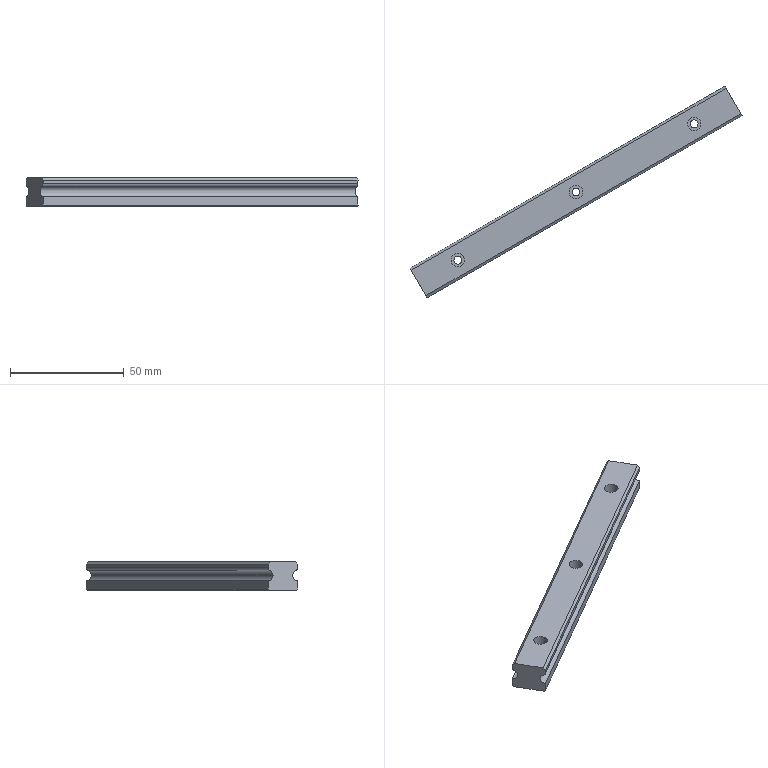Part | SolidWorks | features BaseBody 1 | 1 solid | 32 faces | box 146.064 x 92.99 x 12.5 mm | volume 26238 mm3 | cylinder 17 | plane 15 | commonest cylinder face diameters 3.5 x6 6 x6 4.4 x3 3 x2
STEP:
#1=CARTESIAN_POINT('',(297.681,1789.378,-1208.57));
#2=VERTEX_POINT('',#1);
#3=CARTESIAN_POINT('',(294.181,1789.378,-1208.57));
#4=VERTEX_POINT('',#3);
#5=CARTESIAN_POINT('',(295.931,1789.378,-1208.57));
#6=DIRECTION('',(0.,0.,-1.));
#7=DIRECTION('',(1.,0.,0.));
#8=AXIS2_PLACEMENT_3D('',#5,#6,#7);
#9=CIRCLE('',#8,1.75);
#10=EDGE_CURVE('',#2,#4,#9,.T.);
#11=ORIENTED_EDGE('',*,*,#10,.T.);
#12=CARTESIAN_POINT('',(294.181,1789.378,-1200.57));
#13=VERTEX_POINT('',#12);
#14=CARTESIAN_POINT('',(294.181,1789.378,-1196.07));
#15=DIRECTION('',(0.,0.,1.));
#16=VECTOR('',#15,1000.);
#17=LINE('',#14,#16);
#18=EDGE_CURVE('',#4,#13,#17,.T.);
#19=ORIENTED_EDGE('',*,*,#18,.T.);
#20=CARTESIAN_POINT('',(297.681,1789.378,-1200.57));
#21=VERTEX_POINT('',#20);
#22=CARTESIAN_POINT('',(295.931,1789.378,-1200.57));
#23=DIRECTION('',(0.,0.,-1.));
#24=DIRECTION('',(1.,0.,0.));
#25=AXIS2_PLACEMENT_3D('',#22,#23,#24);
#26=CIRCLE('',#25,1.75);
#27=EDGE_CURVE('',#21,#13,#26,.T.);
#28=ORIENTED_EDGE('',*,*,#27,.F.);
#29=CARTESIAN_POINT('',(297.681,1789.378,-1196.07));
#30=DIRECTION('',(0.,0.,1.));
#31=VECTOR('',#30,1000.);
#32=LINE('',#29,#31);
#33=EDGE_CURVE('',#2,#21,#32,.T.);
#34=ORIENTED_EDGE('',*,*,#33,.F.);
#35=EDGE_LOOP('',(#11,#19,#28,#34));
#36=FACE_OUTER_BOUND('',#35,.T.);
#37=CARTESIAN_POINT('',(295.931,1789.378,-1196.07));
#38=DIRECTION('',(0.,0.,1.));
#39=DIRECTION('',(1.,0.,0.));
#40=AXIS2_PLACEMENT_3D('',#37,#38,#39);
#41=CYLINDRICAL_SURFACE('',#40,1.75);
#42=ADVANCED_FACE('',(#36),#41,.F.);
#43=CARTESIAN_POINT('',(401.604,1849.378,-1208.57));
#44=VERTEX_POINT('',#43);
#45=CARTESIAN_POINT('',(398.104,1849.378,-1208.57));
#46=VERTEX_POINT('',#45);
#47=CARTESIAN_POINT('',(399.854,1849.378,-1208.57));
#48=DIRECTION('',(0.,0.,-1.));
#49=DIRECTION('',(1.,0.,0.));
#50=AXIS2_PLACEMENT_3D('',#47,#48,#49);
#51=CIRCLE('',#50,1.75);
#52=EDGE_CURVE('',#44,#46,#51,.T.);
#53=ORIENTED_EDGE('',*,*,#52,.T.);
#54=CARTESIAN_POINT('',(398.104,1849.378,-1200.57));
#55=VERTEX_POINT('',#54);
#56=CARTESIAN_POINT('',(398.104,1849.378,-1196.07));
#57=DIRECTION('',(0.,0.,1.));
#58=VECTOR('',#57,1000.);
#59=LINE('',#56,#58);
#60=EDGE_CURVE('',#46,#55,#59,.T.);
#61=ORIENTED_EDGE('',*,*,#60,.T.);
#62=CARTESIAN_POINT('',(401.604,1849.378,-1200.57));
#63=VERTEX_POINT('',#62);
#64=CARTESIAN_POINT('',(399.854,1849.378,-1200.57));
#65=DIRECTION('',(0.,0.,-1.));
#66=DIRECTION('',(1.,0.,0.));
#67=AXIS2_PLACEMENT_3D('',#64,#65,#66);
#68=CIRCLE('',#67,1.75);
#69=EDGE_CURVE('',#63,#55,#68,.T.);
#70=ORIENTED_EDGE('',*,*,#69,.F.);
#71=CARTESIAN_POINT('',(401.604,1849.378,-1196.07));
#72=DIRECTION('',(0.,0.,1.));
#73=VECTOR('',#72,1000.);
#74=LINE('',#71,#73);
#75=EDGE_CURVE('',#44,#63,#74,.T.);
#76=ORIENTED_EDGE('',*,*,#75,.F.);
#77=EDGE_LOOP('',(#53,#61,#70,#76));
#78=FACE_OUTER_BOUND('',#77,.T.);
#79=CARTESIAN_POINT('',(399.854,1849.378,-1196.07));
#80=DIRECTION('',(0.,0.,1.));
#81=DIRECTION('',(1.,0.,0.));
#82=AXIS2_PLACEMENT_3D('',#79,#80,#81);
#83=CYLINDRICAL_SURFACE('',#82,1.75);
#84=ADVANCED_FACE('',(#78),#83,.F.);
#85=CARTESIAN_POINT('',(349.643,1819.378,-1208.57));
#86=VERTEX_POINT('',#85);
#87=CARTESIAN_POINT('',(346.143,1819.378,-1208.57));
#88=VERTEX_POINT('',#87);
#89=CARTESIAN_POINT('',(347.893,1819.378,-1208.57));
#90=DIRECTION('',(0.,0.,-1.));
#91=DIRECTION('',(1.,0.,0.));
#92=AXIS2_PLACEMENT_3D('',#89,#90,#91);
#93=CIRCLE('',#92,1.75);
#94=EDGE_CURVE('',#86,#88,#93,.T.);
#95=ORIENTED_EDGE('',*,*,#94,.T.);
#96=CARTESIAN_POINT('',(346.143,1819.378,-1200.57));
#97=VERTEX_POINT('',#96);
#98=CARTESIAN_POINT('',(346.143,1819.378,-1196.07));
#99=DIRECTION('',(0.,0.,1.));
#100=VECTOR('',#99,1000.);
#101=LINE('',#98,#100);
#102=EDGE_CURVE('',#88,#97,#101,.T.);
#103=ORIENTED_EDGE('',*,*,#102,.T.);
#104=CARTESIAN_POINT('',(349.643,1819.378,-1200.57));
#105=VERTEX_POINT('',#104);
#106=CARTESIAN_POINT('',(347.893,1819.378,-1200.57));
#107=DIRECTION('',(0.,0.,-1.));
#108=DIRECTION('',(1.,0.,0.));
#109=AXIS2_PLACEMENT_3D('',#106,#107,#108);
#110=CIRCLE('',#109,1.75);
#111=EDGE_CURVE('',#105,#97,#110,.T.);
#112=ORIENTED_EDGE('',*,*,#111,.F.);
#113=CARTESIAN_POINT('',(349.643,1819.378,-1196.07));
#114=DIRECTION('',(0.,0.,1.));
#115=VECTOR('',#114,1000.);
#116=LINE('',#113,#115);
#117=EDGE_CURVE('',#86,#105,#116,.T.);
#118=ORIENTED_EDGE('',*,*,#117,.F.);
#119=EDGE_LOOP('',(#95,#103,#112,#118));
#120=FACE_OUTER_BOUND('',#119,.T.);
#121=CARTESIAN_POINT('',(347.893,1819.378,-1196.07));
#122=DIRECTION('',(0.,0.,1.));
#123=DIRECTION('',(1.,0.,0.));
#124=AXIS2_PLACEMENT_3D('',#121,#122,#123);
#125=CYLINDRICAL_SURFACE('',#124,1.75);
#126=ADVANCED_FACE('',(#120),#125,.F.);
#127=CARTESIAN_POINT('',(414.675,1863.708,-1202.07));
#128=VERTEX_POINT('',#127);
#129=CARTESIAN_POINT('',(413.932,1864.995,-1199.989));
#130=VERTEX_POINT('',#129);
#131=CARTESIAN_POINT('',(413.575,1865.613,-1202.07));
#132=DIRECTION('',(-0.866,-0.5,0.));
#133=DIRECTION('',(0.5,-0.866,0.));
#134=AXIS2_PLACEMENT_3D('',#131,#132,#133);
#135=CIRCLE('',#134,2.2);
#136=EDGE_CURVE('',#128,#130,#135,.T.);
#137=ORIENTED_EDGE('',*,*,#136,.F.);
#138=CARTESIAN_POINT('',(276.111,1783.708,-1202.07));
#139=VERTEX_POINT('',#138);
#140=CARTESIAN_POINT('',(414.675,1863.708,-1202.07));
#141=DIRECTION('',(-0.866,-0.5,0.));
#142=VECTOR('',#141,1000.);
#143=LINE('',#140,#142);
#144=EDGE_CURVE('',#128,#139,#143,.T.);
#145=ORIENTED_EDGE('',*,*,#144,.T.);
#146=CARTESIAN_POINT('',(275.367,1784.995,-1199.989));
#147=VERTEX_POINT('',#146);
#148=CARTESIAN_POINT('',(275.011,1785.613,-1202.07));
#149=DIRECTION('',(-0.866,-0.5,0.));
#150=DIRECTION('',(0.5,-0.866,0.));
#151=AXIS2_PLACEMENT_3D('',#148,#149,#150);
#152=CIRCLE('',#151,2.2);
#153=EDGE_CURVE('',#139,#147,#152,.T.);
#154=ORIENTED_EDGE('',*,*,#153,.T.);
#155=CARTESIAN_POINT('',(413.932,1864.995,-1199.989));
#156=DIRECTION('',(-0.866,-0.5,0.));
#157=VECTOR('',#156,1000.);
#158=LINE('',#155,#157);
#159=EDGE_CURVE('',#130,#147,#158,.T.);
#160=ORIENTED_EDGE('',*,*,#159,.F.);
#161=EDGE_LOOP('',(#137,#145,#154,#160));
#162=FACE_OUTER_BOUND('',#161,.T.);
#163=CARTESIAN_POINT('',(413.575,1865.613,-1202.07));
#164=DIRECTION('',(-0.866,-0.5,0.));
#165=DIRECTION('',(0.5,-0.866,0.));
#166=AXIS2_PLACEMENT_3D('',#163,#164,#165);
#167=CYLINDRICAL_SURFACE('',#166,2.2);
#168=ADVANCED_FACE('',(#162),#167,.F.);
#169=CARTESIAN_POINT('',(298.931,1789.378,-1200.57));
#170=VERTEX_POINT('',#169);
#171=CARTESIAN_POINT('',(292.931,1789.378,-1200.57));
#172=VERTEX_POINT('',#171);
#173=CARTESIAN_POINT('',(295.931,1789.378,-1200.57));
#174=DIRECTION('',(0.,0.,-1.));
#175=DIRECTION('',(1.,0.,0.));
#176=AXIS2_PLACEMENT_3D('',#173,#174,#175);
#177=CIRCLE('',#176,3.);
#178=EDGE_CURVE('',#170,#172,#177,.T.);
#179=ORIENTED_EDGE('',*,*,#178,.T.);
#180=CARTESIAN_POINT('',(292.931,1789.378,-1196.07));
#181=VERTEX_POINT('',#180);
#182=CARTESIAN_POINT('',(292.931,1789.378,-1196.07));
#183=DIRECTION('',(0.,0.,1.));
#184=VECTOR('',#183,1000.);
#185=LINE('',#182,#184);
#186=EDGE_CURVE('',#172,#181,#185,.T.);
#187=ORIENTED_EDGE('',*,*,#186,.T.);
#188=CARTESIAN_POINT('',(298.931,1789.378,-1196.07));
#189=VERTEX_POINT('',#188);
#190=CARTESIAN_POINT('',(295.931,1789.378,-1196.07));
#191=DIRECTION('',(0.,0.,1.));
#192=DIRECTION('',(1.,0.,0.));
#193=AXIS2_PLACEMENT_3D('',#190,#191,#192);
#194=CIRCLE('',#193,3.);
#195=EDGE_CURVE('',#181,#189,#194,.T.);
#196=ORIENTED_EDGE('',*,*,#195,.T.);
#197=CARTESIAN_POINT('',(298.931,1789.378,-1196.07));
#198=DIRECTION('',(0.,0.,1.));
#199=VECTOR('',#198,1000.);
#200=LINE('',#197,#199);
#201=EDGE_CURVE('',#170,#189,#200,.T.);
#202=ORIENTED_EDGE('',*,*,#201,.F.);
#203=EDGE_LOOP('',(#179,#187,#196,#202));
#204=FACE_OUTER_BOUND('',#203,.T.);
#205=CARTESIAN_POINT('',(295.931,1789.378,-1196.07));
#206=DIRECTION('',(0.,0.,1.));
#207=DIRECTION('',(1.,0.,0.));
#208=AXIS2_PLACEMENT_3D('',#205,#206,#207);
#209=CYLINDRICAL_SURFACE('',#208,3.);
#210=ADVANCED_FACE('',(#204),#209,.F.);
#211=CARTESIAN_POINT('',(402.854,1849.378,-1200.57));
#212=VERTEX_POINT('',#211);
#213=CARTESIAN_POINT('',(396.854,1849.378,-1200.57));
#214=VERTEX_POINT('',#213);
#215=CARTESIAN_POINT('',(399.854,1849.378,-1200.57));
#216=DIRECTION('',(0.,0.,-1.));
#217=DIRECTION('',(1.,0.,0.));
#218=AXIS2_PLACEMENT_3D('',#215,#216,#217);
#219=CIRCLE('',#218,3.);
#220=EDGE_CURVE('',#212,#214,#219,.T.);
#221=ORIENTED_EDGE('',*,*,#220,.T.);
#222=CARTESIAN_POINT('',(396.854,1849.378,-1196.07));
#223=VERTEX_POINT('',#222);
#224=CARTESIAN_POINT('',(396.854,1849.378,-1196.07));
#225=DIRECTION('',(0.,0.,1.));
#226=VECTOR('',#225,1000.);
#227=LINE('',#224,#226);
#228=EDGE_CURVE('',#214,#223,#227,.T.);
#229=ORIENTED_EDGE('',*,*,#228,.T.);
#230=CARTESIAN_POINT('',(402.854,1849.378,-1196.07));
#231=VERTEX_POINT('',#230);
#232=CARTESIAN_POINT('',(399.854,1849.378,-1196.07));
#233=DIRECTION('',(0.,0.,1.));
#234=DIRECTION('',(1.,0.,0.));
#235=AXIS2_PLACEMENT_3D('',#232,#233,#234);
#236=CIRCLE('',#235,3.);
#237=EDGE_CURVE('',#223,#231,#236,.T.);
#238=ORIENTED_EDGE('',*,*,#237,.T.);
#239=CARTESIAN_POINT('',(402.854,1849.378,-1196.07));
#240=DIRECTION('',(0.,0.,1.));
#241=VECTOR('',#240,1000.);
#242=LINE('',#239,#241);
#243=EDGE_CURVE('',#212,#231,#242,.T.);
#244=ORIENTED_EDGE('',*,*,#243,.F.);
#245=EDGE_LOOP('',(#221,#229,#238,#244));
#246=FACE_OUTER_BOUND('',#245,.T.);
#247=CARTESIAN_POINT('',(399.854,1849.378,-1196.07));
#248=DIRECTION('',(0.,0.,1.));
#249=DIRECTION('',(1.,0.,0.));
#250=AXIS2_PLACEMENT_3D('',#247,#248,#249);
#251=CYLINDRICAL_SURFACE('',#250,3.);
#252=ADVANCED_FACE('',(#246),#251,.F.);
#253=CARTESIAN_POINT('',(350.893,1819.378,-1200.57));
#254=VERTEX_POINT('',#253);
#255=CARTESIAN_POINT('',(344.893,1819.378,-1200.57));
#256=VERTEX_POINT('',#255);
#257=CARTESIAN_POINT('',(347.893,1819.378,-1200.57));
#258=DIRECTION('',(0.,0.,-1.));
#259=DIRECTION('',(1.,0.,0.));
#260=AXIS2_PLACEMENT_3D('',#257,#258,#259);
#261=CIRCLE('',#260,3.);
#262=EDGE_CURVE('',#254,#256,#261,.T.);
#263=ORIENTED_EDGE('',*,*,#262,.T.);
#264=CARTESIAN_POINT('',(344.893,1819.378,-1196.07));
#265=VERTEX_POINT('',#264);
#266=CARTESIAN_POINT('',(344.893,1819.378,-1196.07));
#267=DIRECTION('',(0.,0.,1.));
#268=VECTOR('',#267,1000.);
#269=LINE('',#266,#268);
#270=EDGE_CURVE('',#256,#265,#269,.T.);
#271=ORIENTED_EDGE('',*,*,#270,.T.);
#272=CARTESIAN_POINT('',(350.893,1819.378,-1196.07));
#273=VERTEX_POINT('',#272);
#274=CARTESIAN_POINT('',(347.893,1819.378,-1196.07));
#275=DIRECTION('',(0.,0.,1.));
#276=DIRECTION('',(1.,0.,0.));
#277=AXIS2_PLACEMENT_3D('',#274,#275,#276);
#278=CIRCLE('',#277,3.);
#279=EDGE_CURVE('',#265,#273,#278,.T.);
#280=ORIENTED_EDGE('',*,*,#279,.T.);
#281=CARTESIAN_POINT('',(350.893,1819.378,-1196.07));
#282=DIRECTION('',(0.,0.,1.));
#283=VECTOR('',#282,1000.);
#284=LINE('',#281,#283);
#285=EDGE_CURVE('',#254,#273,#284,.T.);
#286=ORIENTED_EDGE('',*,*,#285,.F.);
#287=EDGE_LOOP('',(#263,#271,#280,#286));
#288=FACE_OUTER_BOUND('',#287,.T.);
#289=CARTESIAN_POINT('',(347.893,1819.378,-1196.07));
#290=DIRECTION('',(0.,0.,1.));
#291=DIRECTION('',(1.,0.,0.));
#292=AXIS2_PLACEMENT_3D('',#289,#290,#291);
#293=CYLINDRICAL_SURFACE('',#292,3.);
#294=ADVANCED_FACE('',(#288),#293,.F.);
#295=ORIENTED_EDGE('',*,*,#10,.F.);
#296=CARTESIAN_POINT('',(295.931,1789.378,-1208.57));
#297=DIRECTION('',(0.,0.,-1.));
#298=DIRECTION('',(1.,0.,0.));
#299=AXIS2_PLACEMENT_3D('',#296,#297,#298);
#300=CIRCLE('',#299,1.75);
#301=EDGE_CURVE('',#4,#2,#300,.T.);
#302=ORIENTED_EDGE('',*,*,#301,.F.);
#303=EDGE_LOOP('',(#295,#302));
#304=FACE_BOUND('',#303,.T.);
#305=ORIENTED_EDGE('',*,*,#52,.F.);
#306=CARTESIAN_POINT('',(399.854,1849.378,-1208.57));
#307=DIRECTION('',(0.,0.,-1.));
#308=DIRECTION('',(1.,0.,0.));
#309=AXIS2_PLACEMENT_3D('',#306,#307,#308);
#310=CIRCLE('',#309,1.75);
#311=EDGE_CURVE('',#46,#44,#310,.T.);
#312=ORIENTED_EDGE('',*,*,#311,.F.);
#313=EDGE_LOOP('',(#305,#312));
#314=FACE_BOUND('',#313,.T.);
#315=ORIENTED_EDGE('',*,*,#94,.F.);
#316=CARTESIAN_POINT('',(347.893,1819.378,-1208.57));
#317=DIRECTION('',(0.,0.,-1.));
#318=DIRECTION('',(1.,0.,0.));
#319=AXIS2_PLACEMENT_3D('',#316,#317,#318);
#320=CIRCLE('',#319,1.75);
#321=EDGE_CURVE('',#88,#86,#320,.T.);
#322=ORIENTED_EDGE('',*,*,#321,.F.);
#323=EDGE_LOOP('',(#315,#322));
#324=FACE_BOUND('',#323,.T.);
#325=CARTESIAN_POINT('',(420.675,1853.315,-1208.57));
#326=VERTEX_POINT('',#325);
#327=CARTESIAN_POINT('',(413.675,1865.44,-1208.57));
#328=VERTEX_POINT('',#327);
#329=CARTESIAN_POINT('',(420.675,1853.315,-1208.57));
#330=DIRECTION('',(-0.5,0.866,0.));
#331=VECTOR('',#330,1000.);
#332=LINE('',#329,#331);
#333=EDGE_CURVE('',#326,#328,#332,.T.);
#334=ORIENTED_EDGE('',*,*,#333,.F.);
#335=CARTESIAN_POINT('',(282.111,1773.315,-1208.57));
#336=VERTEX_POINT('',#335);
#337=CARTESIAN_POINT('',(282.111,1773.315,-1208.57));
#338=DIRECTION('',(0.866,0.5,0.));
#339=VECTOR('',#338,1000.);
#340=LINE('',#337,#339);
#341=EDGE_CURVE('',#336,#326,#340,.T.);
#342=ORIENTED_EDGE('',*,*,#341,.F.);
#343=CARTESIAN_POINT('',(275.111,1785.44,-1208.57));
#344=VERTEX_POINT('',#343);
#345=CARTESIAN_POINT('',(275.111,1785.44,-1208.57));
#346=DIRECTION('',(0.5,-0.866,0.));
#347=VECTOR('',#346,1000.);
#348=LINE('',#345,#347);
#349=EDGE_CURVE('',#344,#336,#348,.T.);
#350=ORIENTED_EDGE('',*,*,#349,.F.);
#351=CARTESIAN_POINT('',(413.675,1865.44,-1208.57));
#352=DIRECTION('',(-0.866,-0.5,0.));
#353=VECTOR('',#352,1000.);
#354=LINE('',#351,#353);
#355=EDGE_CURVE('',#328,#344,#354,.T.);
#356=ORIENTED_EDGE('',*,*,#355,.F.);
#357=EDGE_LOOP('',(#334,#342,#350,#356));
#358=FACE_OUTER_BOUND('',#357,.T.);
#359=CARTESIAN_POINT('',(420.675,1853.315,-1208.57));
#360=DIRECTION('',(0.,0.,1.));
#361=DIRECTION('',(1.,0.,0.));
#362=AXIS2_PLACEMENT_3D('',#359,#360,#361);
#363=PLANE('',#362);
#364=ADVANCED_FACE('',(#304,#314,#324,#358),#363,.F.);
#365=ORIENTED_EDGE('',*,*,#18,.F.);
#366=ORIENTED_EDGE('',*,*,#301,.T.);
#367=ORIENTED_EDGE('',*,*,#33,.T.);
#368=CARTESIAN_POINT('',(295.931,1789.378,-1200.57));
#369=DIRECTION('',(0.,0.,-1.));
#370=DIRECTION('',(1.,0.,0.));
#371=AXIS2_PLACEMENT_3D('',#368,#369,#370);
#372=CIRCLE('',#371,1.75);
#373=EDGE_CURVE('',#13,#21,#372,.T.);
#374=ORIENTED_EDGE('',*,*,#373,.F.);
#375=EDGE_LOOP('',(#365,#366,#367,#374));
#376=FACE_OUTER_BOUND('',#375,.T.);
#377=CARTESIAN_POINT('',(295.931,1789.378,-1196.07));
#378=DIRECTION('',(0.,0.,1.));
#379=DIRECTION('',(1.,0.,0.));
#380=AXIS2_PLACEMENT_3D('',#377,#378,#379);
#381=CYLINDRICAL_SURFACE('',#380,1.75);
#382=ADVANCED_FACE('',(#376),#381,.F.);
#383=ORIENTED_EDGE('',*,*,#60,.F.);
#384=ORIENTED_EDGE('',*,*,#311,.T.);
#385=ORIENTED_EDGE('',*,*,#75,.T.);
#386=CARTESIAN_POINT('',(399.854,1849.378,-1200.57));
#387=DIRECTION('',(0.,0.,-1.));
#388=DIRECTION('',(1.,0.,0.));
#389=AXIS2_PLACEMENT_3D('',#386,#387,#388);
#390=CIRCLE('',#389,1.75);
#391=EDGE_CURVE('',#55,#63,#390,.T.);
#392=ORIENTED_EDGE('',*,*,#391,.F.);
#393=EDGE_LOOP('',(#383,#384,#385,#392));
#394=FACE_OUTER_BOUND('',#393,.T.);
#395=CARTESIAN_POINT('',(399.854,1849.378,-1196.07));
#396=DIRECTION('',(0.,0.,1.));
#397=DIRECTION('',(1.,0.,0.));
#398=AXIS2_PLACEMENT_3D('',#395,#396,#397);
#399=CYLINDRICAL_SURFACE('',#398,1.75);
#400=ADVANCED_FACE('',(#394),#399,.F.);
#401=ORIENTED_EDGE('',*,*,#102,.F.);
#402=ORIENTED_EDGE('',*,*,#321,.T.);
#403=ORIENTED_EDGE('',*,*,#117,.T.);
#404=CARTESIAN_POINT('',(347.893,1819.378,-1200.57));
#405=DIRECTION('',(0.,0.,-1.));
#406=DIRECTION('',(1.,0.,0.));
#407=AXIS2_PLACEMENT_3D('',#404,#405,#406);
#408=CIRCLE('',#407,1.75);
#409=EDGE_CURVE('',#97,#105,#408,.T.);
#410=ORIENTED_EDGE('',*,*,#409,.F.);
#411=EDGE_LOOP('',(#401,#402,#403,#410));
#412=FACE_OUTER_BOUND('',#411,.T.);
#413=CARTESIAN_POINT('',(347.893,1819.378,-1196.07));
#414=DIRECTION('',(0.,0.,1.));
#415=DIRECTION('',(1.,0.,0.));
#416=AXIS2_PLACEMENT_3D('',#413,#414,#415);
#417=CYLINDRICAL_SURFACE('',#416,1.75);
#418=ADVANCED_FACE('',(#412),#417,.F.);
#419=CARTESIAN_POINT('',(413.425,1865.873,-1208.07));
#420=VERTEX_POINT('',#419);
#421=CARTESIAN_POINT('',(413.675,1865.44,-1208.57));
#422=DIRECTION('',(-0.3536,0.6124,0.7071));
#423=VECTOR('',#422,1000.);
#424=LINE('',#421,#423);
#425=EDGE_CURVE('',#328,#420,#424,.T.);
#426=ORIENTED_EDGE('',*,*,#425,.F.);
#427=ORIENTED_EDGE('',*,*,#355,.T.);
#428=CARTESIAN_POINT('',(274.861,1785.873,-1208.07));
#429=VERTEX_POINT('',#428);
#430=CARTESIAN_POINT('',(274.861,1785.873,-1208.07));
#431=DIRECTION('',(0.3536,-0.6124,-0.7071));
#432=VECTOR('',#431,1000.);
#433=LINE('',#430,#432);
#434=EDGE_CURVE('',#429,#344,#433,.T.);
#435=ORIENTED_EDGE('',*,*,#434,.F.);
#436=CARTESIAN_POINT('',(413.425,1865.873,-1208.07));
#437=DIRECTION('',(-0.866,-0.5,0.));
#438=VECTOR('',#437,1000.);
#439=LINE('',#436,#438);
#440=EDGE_CURVE('',#420,#429,#439,.T.);
#441=ORIENTED_EDGE('',*,*,#440,.F.);
#442=EDGE_LOOP('',(#426,#427,#435,#441));
#443=FACE_OUTER_BOUND('',#442,.T.);
#444=CARTESIAN_POINT('',(413.425,1865.873,-1208.07));
#445=DIRECTION('',(0.3536,-0.6124,0.7071));
#446=DIRECTION('',(0.,-0.7559,-0.6547));
#447=AXIS2_PLACEMENT_3D('',#444,#445,#446);
#448=PLANE('',#447);
#449=ADVANCED_FACE('',(#443),#448,.F.);
#450=CARTESIAN_POINT('',(413.425,1865.873,-1197.07));
#451=VERTEX_POINT('',#450);
#452=CARTESIAN_POINT('',(413.925,1865.007,-1196.07));
#453=VERTEX_POINT('',#452);
#454=CARTESIAN_POINT('',(413.425,1865.873,-1197.07));
#455=DIRECTION('',(0.3536,-0.6124,0.7071));
#456=VECTOR('',#455,1000.);
#457=LINE('',#454,#456);
#458=EDGE_CURVE('',#451,#453,#457,.T.);
#459=ORIENTED_EDGE('',*,*,#458,.T.);
#460=CARTESIAN_POINT('',(420.425,1853.748,-1196.07));
#461=VERTEX_POINT('',#460);
#462=CARTESIAN_POINT('',(420.175,1854.181,-1196.07));
#463=DIRECTION('',(0.5,-0.866,0.));
#464=VECTOR('',#463,1000.);
#465=LINE('',#462,#464);
#466=EDGE_CURVE('',#453,#461,#465,.T.);
#467=ORIENTED_EDGE('',*,*,#466,.T.);
#468=CARTESIAN_POINT('',(420.925,1852.882,-1197.07));
#469=VERTEX_POINT('',#468);
#470=CARTESIAN_POINT('',(420.425,1853.748,-1196.07));
#471=DIRECTION('',(0.3536,-0.6124,-0.7071));
#472=VECTOR('',#471,1000.);
#473=LINE('',#470,#472);
#474=EDGE_CURVE('',#461,#469,#473,.T.);
#475=ORIENTED_EDGE('',*,*,#474,.T.);
#476=CARTESIAN_POINT('',(420.925,1852.882,-1198.57));
#477=VERTEX_POINT('',#476);
#478=CARTESIAN_POINT('',(420.925,1852.882,-1198.57));
#479=DIRECTION('',(0.,0.,-1.));
#480=VECTOR('',#479,1000.);
#481=LINE('',#478,#480);
#482=EDGE_CURVE('',#469,#477,#481,.T.);
#483=ORIENTED_EDGE('',*,*,#482,.T.);
#484=CARTESIAN_POINT('',(420.418,1853.76,-1199.989));
#485=VERTEX_POINT('',#484);
#486=CARTESIAN_POINT('',(420.175,1854.181,-1198.57));
#487=DIRECTION('',(0.866,0.5,0.));
#488=DIRECTION('',(0.5,-0.866,0.));
#489=AXIS2_PLACEMENT_3D('',#486,#487,#488);
#490=CIRCLE('',#489,1.5);
#491=EDGE_CURVE('',#477,#485,#490,.T.);
#492=ORIENTED_EDGE('',*,*,#491,.T.);
#493=CARTESIAN_POINT('',(420.925,1852.882,-1204.249));
#494=VERTEX_POINT('',#493);
#495=CARTESIAN_POINT('',(420.775,1853.142,-1202.07));
#496=DIRECTION('',(-0.866,-0.5,0.));
#497=DIRECTION('',(0.5,-0.866,0.));
#498=AXIS2_PLACEMENT_3D('',#495,#496,#497);
#499=CIRCLE('',#498,2.2);
#500=EDGE_CURVE('',#485,#494,#499,.T.);
#501=ORIENTED_EDGE('',*,*,#500,.T.);
#502=CARTESIAN_POINT('',(420.925,1852.882,-1208.07));
#503=VERTEX_POINT('',#502);
#504=CARTESIAN_POINT('',(420.925,1852.882,-1198.57));
#505=DIRECTION('',(0.,0.,-1.));
#506=VECTOR('',#505,1000.);
#507=LINE('',#504,#506);
#508=EDGE_CURVE('',#494,#503,#507,.T.);
#509=ORIENTED_EDGE('',*,*,#508,.T.);
#510=CARTESIAN_POINT('',(420.925,1852.882,-1208.07));
#511=DIRECTION('',(-0.3536,0.6124,-0.7071));
#512=VECTOR('',#511,1000.);
#513=LINE('',#510,#512);
#514=EDGE_CURVE('',#503,#326,#513,.T.);
#515=ORIENTED_EDGE('',*,*,#514,.T.);
#516=ORIENTED_EDGE('',*,*,#333,.T.);
#517=ORIENTED_EDGE('',*,*,#425,.T.);
#518=CARTESIAN_POINT('',(413.425,1865.873,-1204.249));
#519=VERTEX_POINT('',#518);
#520=CARTESIAN_POINT('',(413.425,1865.873,-1198.57));
#521=DIRECTION('',(0.,0.,1.));
#522=VECTOR('',#521,1000.);
#523=LINE('',#520,#522);
#524=EDGE_CURVE('',#420,#519,#523,.T.);
#525=ORIENTED_EDGE('',*,*,#524,.T.);
#526=CARTESIAN_POINT('',(413.575,1865.613,-1202.07));
#527=DIRECTION('',(-0.866,-0.5,0.));
#528=DIRECTION('',(0.5,-0.866,0.));
#529=AXIS2_PLACEMENT_3D('',#526,#527,#528);
#530=CIRCLE('',#529,2.2);
#531=EDGE_CURVE('',#519,#128,#530,.T.);
#532=ORIENTED_EDGE('',*,*,#531,.T.);
#533=ORIENTED_EDGE('',*,*,#136,.T.);
#534=CARTESIAN_POINT('',(413.425,1865.873,-1198.57));
#535=VERTEX_POINT('',#534);
#536=CARTESIAN_POINT('',(414.175,1864.574,-1198.57));
#537=DIRECTION('',(0.866,0.5,0.));
#538=DIRECTION('',(0.5,-0.866,0.));
#539=AXIS2_PLACEMENT_3D('',#536,#537,#538);
#540=CIRCLE('',#539,1.5);
#541=EDGE_CURVE('',#130,#535,#540,.T.);
#542=ORIENTED_EDGE('',*,*,#541,.T.);
#543=CARTESIAN_POINT('',(413.425,1865.873,-1198.57));
#544=DIRECTION('',(0.,0.,1.));
#545=VECTOR('',#544,1000.);
#546=LINE('',#543,#545);
#547=EDGE_CURVE('',#535,#451,#546,.T.);
#548=ORIENTED_EDGE('',*,*,#547,.T.);
#549=EDGE_LOOP('',(#459,#467,#475,#483,#492,#501,#509,#515,#516,#517,#525,#532,#533,#542,#548));
#550=FACE_OUTER_BOUND('',#549,.T.);
#551=CARTESIAN_POINT('',(420.175,1854.181,-1198.57));
#552=DIRECTION('',(0.866,0.5,0.));
#553=DIRECTION('',(-0.5,0.866,0.));
#554=AXIS2_PLACEMENT_3D('',#551,#552,#553);
#555=PLANE('',#554);
#556=ADVANCED_FACE('',(#550),#555,.T.);
#557=ORIENTED_EDGE('',*,*,#514,.F.);
#558=CARTESIAN_POINT('',(282.361,1772.882,-1208.07));
#559=VERTEX_POINT('',#558);
#560=CARTESIAN_POINT('',(282.361,1772.882,-1208.07));
#561=DIRECTION('',(0.866,0.5,0.));
#562=VECTOR('',#561,1000.);
#563=LINE('',#560,#562);
#564=EDGE_CURVE('',#559,#503,#563,.T.);
#565=ORIENTED_EDGE('',*,*,#564,.F.);
#566=CARTESIAN_POINT('',(282.111,1773.315,-1208.57));
#567=DIRECTION('',(0.3536,-0.6124,0.7071));
#568=VECTOR('',#567,1000.);
#569=LINE('',#566,#568);
#570=EDGE_CURVE('',#336,#559,#569,.T.);
#571=ORIENTED_EDGE('',*,*,#570,.F.);
#572=ORIENTED_EDGE('',*,*,#341,.T.);
#573=EDGE_LOOP('',(#557,#565,#571,#572));
#574=FACE_OUTER_BOUND('',#573,.T.);
#575=CARTESIAN_POINT('',(420.925,1852.882,-1208.07));
#576=DIRECTION('',(-0.3536,0.6124,0.7071));
#577=DIRECTION('',(0.,-0.7559,0.6547));
#578=AXIS2_PLACEMENT_3D('',#575,#576,#577);
#579=PLANE('',#578);
#580=ADVANCED_FACE('',(#574),#579,.F.);
#581=CARTESIAN_POINT('',(274.861,1785.873,-1198.57));
#582=VERTEX_POINT('',#581);
#583=CARTESIAN_POINT('',(274.861,1785.873,-1197.07));
#584=VERTEX_POINT('',#583);
#585=CARTESIAN_POINT('',(274.861,1785.873,-1198.57));
#586=DIRECTION('',(0.,0.,1.));
#587=VECTOR('',#586,1000.);
#588=LINE('',#585,#587);
#589=EDGE_CURVE('',#582,#584,#588,.T.);
#590=ORIENTED_EDGE('',*,*,#589,.F.);
#591=CARTESIAN_POINT('',(275.611,1784.574,-1198.57));
#592=DIRECTION('',(0.866,0.5,0.));
#593=DIRECTION('',(0.5,-0.866,0.));
#594=AXIS2_PLACEMENT_3D('',#591,#592,#593);
#595=CIRCLE('',#594,1.5);
#596=EDGE_CURVE('',#147,#582,#595,.T.);
#597=ORIENTED_EDGE('',*,*,#596,.F.);
#598=ORIENTED_EDGE('',*,*,#153,.F.);
#599=CARTESIAN_POINT('',(274.861,1785.873,-1204.249));
#600=VERTEX_POINT('',#599);
#601=CARTESIAN_POINT('',(275.011,1785.613,-1202.07));
#602=DIRECTION('',(-0.866,-0.5,0.));
#603=DIRECTION('',(0.5,-0.866,0.));
#604=AXIS2_PLACEMENT_3D('',#601,#602,#603);
#605=CIRCLE('',#604,2.2);
#606=EDGE_CURVE('',#600,#139,#605,.T.);
#607=ORIENTED_EDGE('',*,*,#606,.F.);
#608=CARTESIAN_POINT('',(274.861,1785.873,-1198.57));
#609=DIRECTION('',(0.,0.,1.));
#610=VECTOR('',#609,1000.);
#611=LINE('',#608,#610);
#612=EDGE_CURVE('',#429,#600,#611,.T.);
#613=ORIENTED_EDGE('',*,*,#612,.F.);
#614=ORIENTED_EDGE('',*,*,#434,.T.);
#615=ORIENTED_EDGE('',*,*,#349,.T.);
#616=ORIENTED_EDGE('',*,*,#570,.T.);
#617=CARTESIAN_POINT('',(282.361,1772.882,-1204.249));
#618=VERTEX_POINT('',#617);
#619=CARTESIAN_POINT('',(282.361,1772.882,-1198.57));
#620=DIRECTION('',(0.,0.,-1.));
#621=VECTOR('',#620,1000.);
#622=LINE('',#619,#621);
#623=EDGE_CURVE('',#618,#559,#622,.T.);
#624=ORIENTED_EDGE('',*,*,#623,.F.);
#625=CARTESIAN_POINT('',(281.854,1773.76,-1199.989));
#626=VERTEX_POINT('',#625);
#627=CARTESIAN_POINT('',(282.211,1773.142,-1202.07));
#628=DIRECTION('',(-0.866,-0.5,0.));
#629=DIRECTION('',(0.5,-0.866,0.));
#630=AXIS2_PLACEMENT_3D('',#627,#628,#629);
#631=CIRCLE('',#630,2.2);
#632=EDGE_CURVE('',#626,#618,#631,.T.);
#633=ORIENTED_EDGE('',*,*,#632,.F.);
#634=CARTESIAN_POINT('',(282.361,1772.882,-1198.57));
#635=VERTEX_POINT('',#634);
#636=CARTESIAN_POINT('',(281.611,1774.181,-1198.57));
#637=DIRECTION('',(0.866,0.5,0.));
#638=DIRECTION('',(0.5,-0.866,0.));
#639=AXIS2_PLACEMENT_3D('',#636,#637,#638);
#640=CIRCLE('',#639,1.5);
#641=EDGE_CURVE('',#635,#626,#640,.T.);
#642=ORIENTED_EDGE('',*,*,#641,.F.);
#643=CARTESIAN_POINT('',(282.361,1772.882,-1197.07));
#644=VERTEX_POINT('',#643);
#645=CARTESIAN_POINT('',(282.361,1772.882,-1198.57));
#646=DIRECTION('',(0.,0.,-1.));
#647=VECTOR('',#646,1000.);
#648=LINE('',#645,#647);
#649=EDGE_CURVE('',#644,#635,#648,.T.);
#650=ORIENTED_EDGE('',*,*,#649,.F.);
#651=CARTESIAN_POINT('',(281.861,1773.748,-1196.07));
#652=VERTEX_POINT('',#651);
#653=CARTESIAN_POINT('',(281.861,1773.748,-1196.07));
#654=DIRECTION('',(0.3536,-0.6124,-0.7071));
#655=VECTOR('',#654,1000.);
#656=LINE('',#653,#655);
#657=EDGE_CURVE('',#652,#644,#656,.T.);
#658=ORIENTED_EDGE('',*,*,#657,.F.);
#659=CARTESIAN_POINT('',(275.361,1785.007,-1196.07));
#660=VERTEX_POINT('',#659);
#661=CARTESIAN_POINT('',(281.611,1774.181,-1196.07));
#662=DIRECTION('',(0.5,-0.866,0.));
#663=VECTOR('',#662,1000.);
#664=LINE('',#661,#663);
#665=EDGE_CURVE('',#660,#652,#664,.T.);
#666=ORIENTED_EDGE('',*,*,#665,.F.);
#667=CARTESIAN_POINT('',(274.861,1785.873,-1197.07));
#668=DIRECTION('',(0.3536,-0.6124,0.7071));
#669=VECTOR('',#668,1000.);
#670=LINE('',#667,#669);
#671=EDGE_CURVE('',#584,#660,#670,.T.);
#672=ORIENTED_EDGE('',*,*,#671,.F.);
#673=EDGE_LOOP('',(#590,#597,#598,#607,#613,#614,#615,#616,#624,#633,#642,#650,#658,#666,#672));
#674=FACE_OUTER_BOUND('',#673,.T.);
#675=CARTESIAN_POINT('',(281.611,1774.181,-1198.57));
#676=DIRECTION('',(0.866,0.5,0.));
#677=DIRECTION('',(-0.5,0.866,0.));
#678=AXIS2_PLACEMENT_3D('',#675,#676,#677);
#679=PLANE('',#678);
#680=ADVANCED_FACE('',(#674),#679,.F.);
#681=ORIENTED_EDGE('',*,*,#27,.T.);
#682=ORIENTED_EDGE('',*,*,#373,.T.);
#683=EDGE_LOOP('',(#681,#682));
#684=FACE_BOUND('',#683,.T.);
#685=ORIENTED_EDGE('',*,*,#178,.F.);
#686=CARTESIAN_POINT('',(295.931,1789.378,-1200.57));
#687=DIRECTION('',(0.,0.,-1.));
#688=DIRECTION('',(1.,0.,0.));
#689=AXIS2_PLACEMENT_3D('',#686,#687,#688);
#690=CIRCLE('',#689,3.);
#691=EDGE_CURVE('',#172,#170,#690,.T.);
#692=ORIENTED_EDGE('',*,*,#691,.F.);
#693=EDGE_LOOP('',(#685,#692));
#694=FACE_OUTER_BOUND('',#693,.T.);
#695=CARTESIAN_POINT('',(297.447,1790.253,-1200.57));
#696=DIRECTION('',(0.,0.,-1.));
#697=DIRECTION('',(-1.,0.,0.));
#698=AXIS2_PLACEMENT_3D('',#695,#696,#697);
#699=PLANE('',#698);
#700=ADVANCED_FACE('',(#684,#694),#699,.F.);
#701=ORIENTED_EDGE('',*,*,#69,.T.);
#702=ORIENTED_EDGE('',*,*,#391,.T.);
#703=EDGE_LOOP('',(#701,#702));
#704=FACE_BOUND('',#703,.T.);
#705=ORIENTED_EDGE('',*,*,#220,.F.);
#706=CARTESIAN_POINT('',(399.854,1849.378,-1200.57));
#707=DIRECTION('',(0.,0.,-1.));
#708=DIRECTION('',(1.,0.,0.));
#709=AXIS2_PLACEMENT_3D('',#706,#707,#708);
#710=CIRCLE('',#709,3.);
#711=EDGE_CURVE('',#214,#212,#710,.T.);
#712=ORIENTED_EDGE('',*,*,#711,.F.);
#713=EDGE_LOOP('',(#705,#712));
#714=FACE_OUTER_BOUND('',#713,.T.);
#715=CARTESIAN_POINT('',(401.37,1850.253,-1200.57));
#716=DIRECTION('',(0.,0.,-1.));
#717=DIRECTION('',(-1.,0.,0.));
#718=AXIS2_PLACEMENT_3D('',#715,#716,#717);
#719=PLANE('',#718);
#720=ADVANCED_FACE('',(#704,#714),#719,.F.);
#721=ORIENTED_EDGE('',*,*,#111,.T.);
#722=ORIENTED_EDGE('',*,*,#409,.T.);
#723=EDGE_LOOP('',(#721,#722));
#724=FACE_BOUND('',#723,.T.);
#725=ORIENTED_EDGE('',*,*,#262,.F.);
#726=CARTESIAN_POINT('',(347.893,1819.378,-1200.57));
#727=DIRECTION('',(0.,0.,-1.));
#728=DIRECTION('',(1.,0.,0.));
#729=AXIS2_PLACEMENT_3D('',#726,#727,#728);
#730=CIRCLE('',#729,3.);
#731=EDGE_CURVE('',#256,#254,#730,.T.);
#732=ORIENTED_EDGE('',*,*,#731,.F.);
#733=EDGE_LOOP('',(#725,#732));
#734=FACE_OUTER_BOUND('',#733,.T.);
#735=CARTESIAN_POINT('',(349.408,1820.253,-1200.57));
#736=DIRECTION('',(0.,0.,-1.));
#737=DIRECTION('',(-1.,0.,0.));
#738=AXIS2_PLACEMENT_3D('',#735,#736,#737);
#739=PLANE('',#738);
#740=ADVANCED_FACE('',(#724,#734),#739,.F.);
#741=ORIENTED_EDGE('',*,*,#524,.F.);
#742=ORIENTED_EDGE('',*,*,#440,.T.);
#743=ORIENTED_EDGE('',*,*,#612,.T.);
#744=CARTESIAN_POINT('',(413.425,1865.873,-1204.249));
#745=DIRECTION('',(-0.866,-0.5,0.));
#746=VECTOR('',#745,1000.);
#747=LINE('',#744,#746);
#748=EDGE_CURVE('',#519,#600,#747,.T.);
#749=ORIENTED_EDGE('',*,*,#748,.F.);
#750=EDGE_LOOP('',(#741,#742,#743,#749));
#751=FACE_OUTER_BOUND('',#750,.T.);
#752=CARTESIAN_POINT('',(413.425,1865.873,-1204.249));
#753=DIRECTION('',(0.5,-0.866,0.));
#754=DIRECTION('',(0.866,0.5,0.));
#755=AXIS2_PLACEMENT_3D('',#752,#753,#754);
#756=PLANE('',#755);
#757=ADVANCED_FACE('',(#751),#756,.F.);
#758=CARTESIAN_POINT('',(295.931,1789.378,-1196.07));
#759=DIRECTION('',(0.,0.,1.));
#760=DIRECTION('',(1.,0.,0.));
#761=AXIS2_PLACEMENT_3D('',#758,#759,#760);
#762=CIRCLE('',#761,3.);
#763=EDGE_CURVE('',#189,#181,#762,.T.);
#764=ORIENTED_EDGE('',*,*,#763,.F.);
#765=ORIENTED_EDGE('',*,*,#195,.F.);
#766=EDGE_LOOP('',(#764,#765));
#767=FACE_BOUND('',#766,.T.);
#768=CARTESIAN_POINT('',(399.854,1849.378,-1196.07));
#769=DIRECTION('',(0.,0.,1.));
#770=DIRECTION('',(1.,0.,0.));
#771=AXIS2_PLACEMENT_3D('',#768,#769,#770);
#772=CIRCLE('',#771,3.);
#773=EDGE_CURVE('',#231,#223,#772,.T.);
#774=ORIENTED_EDGE('',*,*,#773,.F.);
#775=ORIENTED_EDGE('',*,*,#237,.F.);
#776=EDGE_LOOP('',(#774,#775));
#777=FACE_BOUND('',#776,.T.);
#778=CARTESIAN_POINT('',(347.893,1819.378,-1196.07));
#779=DIRECTION('',(0.,0.,1.));
#780=DIRECTION('',(1.,0.,0.));
#781=AXIS2_PLACEMENT_3D('',#778,#779,#780);
#782=CIRCLE('',#781,3.);
#783=EDGE_CURVE('',#273,#265,#782,.T.);
#784=ORIENTED_EDGE('',*,*,#783,.F.);
#785=ORIENTED_EDGE('',*,*,#279,.F.);
#786=EDGE_LOOP('',(#784,#785));
#787=FACE_BOUND('',#786,.T.);
#788=ORIENTED_EDGE('',*,*,#466,.F.);
#789=CARTESIAN_POINT('',(275.361,1785.007,-1196.07));
#790=DIRECTION('',(0.866,0.5,0.));
#791=VECTOR('',#790,1000.);
#792=LINE('',#789,#791);
#793=EDGE_CURVE('',#660,#453,#792,.T.);
#794=ORIENTED_EDGE('',*,*,#793,.F.);
#795=ORIENTED_EDGE('',*,*,#665,.T.);
#796=CARTESIAN_POINT('',(420.425,1853.748,-1196.07));
#797=DIRECTION('',(-0.866,-0.5,0.));
#798=VECTOR('',#797,1000.);
#799=LINE('',#796,#798);
#800=EDGE_CURVE('',#461,#652,#799,.T.);
#801=ORIENTED_EDGE('',*,*,#800,.F.);
#802=EDGE_LOOP('',(#788,#794,#795,#801));
#803=FACE_OUTER_BOUND('',#802,.T.);
#804=CARTESIAN_POINT('',(413.925,1865.007,-1196.07));
#805=DIRECTION('',(0.,0.,-1.));
#806=DIRECTION('',(-1.,0.,0.));
#807=AXIS2_PLACEMENT_3D('',#804,#805,#806);
#808=PLANE('',#807);
#809=ADVANCED_FACE('',(#767,#777,#787,#803),#808,.F.);
#810=ORIENTED_EDGE('',*,*,#458,.F.);
#811=CARTESIAN_POINT('',(274.861,1785.873,-1197.07));
#812=DIRECTION('',(0.866,0.5,0.));
#813=VECTOR('',#812,1000.);
#814=LINE('',#811,#813);
#815=EDGE_CURVE('',#584,#451,#814,.T.);
#816=ORIENTED_EDGE('',*,*,#815,.F.);
#817=ORIENTED_EDGE('',*,*,#671,.T.);
#818=ORIENTED_EDGE('',*,*,#793,.T.);
#819=EDGE_LOOP('',(#810,#816,#817,#818));
#820=FACE_OUTER_BOUND('',#819,.T.);
#821=CARTESIAN_POINT('',(413.925,1865.007,-1196.07));
#822=DIRECTION('',(0.3536,-0.6124,-0.7071));
#823=DIRECTION('',(0.,0.7559,-0.6547));
#824=AXIS2_PLACEMENT_3D('',#821,#822,#823);
#825=PLANE('',#824);
#826=ADVANCED_FACE('',(#820),#825,.F.);
#827=ORIENTED_EDGE('',*,*,#547,.F.);
#828=CARTESIAN_POINT('',(413.425,1865.873,-1198.57));
#829=DIRECTION('',(0.866,0.5,0.));
#830=VECTOR('',#829,1000.);
#831=LINE('',#828,#830);
#832=EDGE_CURVE('',#582,#535,#831,.T.);
#833=ORIENTED_EDGE('',*,*,#832,.F.);
#834=ORIENTED_EDGE('',*,*,#589,.T.);
#835=ORIENTED_EDGE('',*,*,#815,.T.);
#836=EDGE_LOOP('',(#827,#833,#834,#835));
#837=FACE_OUTER_BOUND('',#836,.T.);
#838=CARTESIAN_POINT('',(413.425,1865.873,-1197.07));
#839=DIRECTION('',(0.5,-0.866,0.));
#840=DIRECTION('',(0.866,0.5,0.));
#841=AXIS2_PLACEMENT_3D('',#838,#839,#840);
#842=PLANE('',#841);
#843=ADVANCED_FACE('',(#837),#842,.F.);
#844=ORIENTED_EDGE('',*,*,#159,.T.);
#845=ORIENTED_EDGE('',*,*,#596,.T.);
#846=ORIENTED_EDGE('',*,*,#832,.T.);
#847=ORIENTED_EDGE('',*,*,#541,.F.);
#848=EDGE_LOOP('',(#844,#845,#846,#847));
#849=FACE_OUTER_BOUND('',#848,.T.);
#850=CARTESIAN_POINT('',(414.175,1864.574,-1198.57));
#851=DIRECTION('',(-0.866,-0.5,0.));
#852=DIRECTION('',(0.5,-0.866,0.));
#853=AXIS2_PLACEMENT_3D('',#850,#851,#852);
#854=CYLINDRICAL_SURFACE('',#853,1.5);
#855=ADVANCED_FACE('',(#849),#854,.T.);
#856=ORIENTED_EDGE('',*,*,#144,.F.);
#857=ORIENTED_EDGE('',*,*,#531,.F.);
#858=ORIENTED_EDGE('',*,*,#748,.T.);
#859=ORIENTED_EDGE('',*,*,#606,.T.);
#860=EDGE_LOOP('',(#856,#857,#858,#859));
#861=FACE_OUTER_BOUND('',#860,.T.);
#862=CARTESIAN_POINT('',(413.575,1865.613,-1202.07));
#863=DIRECTION('',(-0.866,-0.5,0.));
#864=DIRECTION('',(0.5,-0.866,0.));
#865=AXIS2_PLACEMENT_3D('',#862,#863,#864);
#866=CYLINDRICAL_SURFACE('',#865,2.2);
#867=ADVANCED_FACE('',(#861),#866,.F.);
#868=ORIENTED_EDGE('',*,*,#508,.F.);
#869=CARTESIAN_POINT('',(420.925,1852.882,-1204.249));
#870=DIRECTION('',(0.866,0.5,0.));
#871=VECTOR('',#870,1000.);
#872=LINE('',#869,#871);
#873=EDGE_CURVE('',#618,#494,#872,.T.);
#874=ORIENTED_EDGE('',*,*,#873,.F.);
#875=ORIENTED_EDGE('',*,*,#623,.T.);
#876=ORIENTED_EDGE('',*,*,#564,.T.);
#877=EDGE_LOOP('',(#868,#874,#875,#876));
#878=FACE_OUTER_BOUND('',#877,.T.);
#879=CARTESIAN_POINT('',(420.925,1852.882,-1204.249));
#880=DIRECTION('',(-0.5,0.866,0.));
#881=DIRECTION('',(-0.866,-0.5,0.));
#882=AXIS2_PLACEMENT_3D('',#879,#880,#881);
#883=PLANE('',#882);
#884=ADVANCED_FACE('',(#878),#883,.F.);
#885=ORIENTED_EDGE('',*,*,#500,.F.);
#886=CARTESIAN_POINT('',(420.418,1853.76,-1199.989));
#887=DIRECTION('',(0.866,0.5,0.));
#888=VECTOR('',#887,1000.);
#889=LINE('',#886,#888);
#890=EDGE_CURVE('',#626,#485,#889,.T.);
#891=ORIENTED_EDGE('',*,*,#890,.F.);
#892=ORIENTED_EDGE('',*,*,#632,.T.);
#893=ORIENTED_EDGE('',*,*,#873,.T.);
#894=EDGE_LOOP('',(#885,#891,#892,#893));
#895=FACE_OUTER_BOUND('',#894,.T.);
#896=CARTESIAN_POINT('',(420.775,1853.142,-1202.07));
#897=DIRECTION('',(-0.866,-0.5,0.));
#898=DIRECTION('',(0.5,-0.866,0.));
#899=AXIS2_PLACEMENT_3D('',#896,#897,#898);
#900=CYLINDRICAL_SURFACE('',#899,2.2);
#901=ADVANCED_FACE('',(#895),#900,.F.);
#902=CARTESIAN_POINT('',(420.925,1852.882,-1198.57));
#903=DIRECTION('',(-0.866,-0.5,0.));
#904=VECTOR('',#903,1000.);
#905=LINE('',#902,#904);
#906=EDGE_CURVE('',#477,#635,#905,.T.);
#907=ORIENTED_EDGE('',*,*,#906,.T.);
#908=ORIENTED_EDGE('',*,*,#641,.T.);
#909=ORIENTED_EDGE('',*,*,#890,.T.);
#910=ORIENTED_EDGE('',*,*,#491,.F.);
#911=EDGE_LOOP('',(#907,#908,#909,#910));
#912=FACE_OUTER_BOUND('',#911,.T.);
#913=CARTESIAN_POINT('',(420.175,1854.181,-1198.57));
#914=DIRECTION('',(-0.866,-0.5,0.));
#915=DIRECTION('',(0.5,-0.866,0.));
#916=AXIS2_PLACEMENT_3D('',#913,#914,#915);
#917=CYLINDRICAL_SURFACE('',#916,1.5);
#918=ADVANCED_FACE('',(#912),#917,.T.);
#919=ORIENTED_EDGE('',*,*,#482,.F.);
#920=CARTESIAN_POINT('',(420.925,1852.882,-1197.07));
#921=DIRECTION('',(0.866,0.5,0.));
#922=VECTOR('',#921,1000.);
#923=LINE('',#920,#922);
#924=EDGE_CURVE('',#644,#469,#923,.T.);
#925=ORIENTED_EDGE('',*,*,#924,.F.);
#926=ORIENTED_EDGE('',*,*,#649,.T.);
#927=ORIENTED_EDGE('',*,*,#906,.F.);
#928=EDGE_LOOP('',(#919,#925,#926,#927));
#929=FACE_OUTER_BOUND('',#928,.T.);
#930=CARTESIAN_POINT('',(420.925,1852.882,-1197.07));
#931=DIRECTION('',(-0.5,0.866,0.));
#932=DIRECTION('',(-0.866,-0.5,0.));
#933=AXIS2_PLACEMENT_3D('',#930,#931,#932);
#934=PLANE('',#933);
#935=ADVANCED_FACE('',(#929),#934,.F.);
#936=ORIENTED_EDGE('',*,*,#474,.F.);
#937=ORIENTED_EDGE('',*,*,#800,.T.);
#938=ORIENTED_EDGE('',*,*,#657,.T.);
#939=ORIENTED_EDGE('',*,*,#924,.T.);
#940=EDGE_LOOP('',(#936,#937,#938,#939));
#941=FACE_OUTER_BOUND('',#940,.T.);
#942=CARTESIAN_POINT('',(420.425,1853.748,-1196.07));
#943=DIRECTION('',(-0.3536,0.6124,-0.7071));
#944=DIRECTION('',(0.,0.7559,0.6547));
#945=AXIS2_PLACEMENT_3D('',#942,#943,#944);
#946=PLANE('',#945);
#947=ADVANCED_FACE('',(#941),#946,.F.);
#948=ORIENTED_EDGE('',*,*,#186,.F.);
#949=ORIENTED_EDGE('',*,*,#691,.T.);
#950=ORIENTED_EDGE('',*,*,#201,.T.);
#951=ORIENTED_EDGE('',*,*,#763,.T.);
#952=EDGE_LOOP('',(#948,#949,#950,#951));
#953=FACE_OUTER_BOUND('',#952,.T.);
#954=CARTESIAN_POINT('',(295.931,1789.378,-1196.07));
#955=DIRECTION('',(0.,0.,1.));
#956=DIRECTION('',(1.,0.,0.));
#957=AXIS2_PLACEMENT_3D('',#954,#955,#956);
#958=CYLINDRICAL_SURFACE('',#957,3.);
#959=ADVANCED_FACE('',(#953),#958,.F.);
#960=ORIENTED_EDGE('',*,*,#228,.F.);
#961=ORIENTED_EDGE('',*,*,#711,.T.);
#962=ORIENTED_EDGE('',*,*,#243,.T.);
#963=ORIENTED_EDGE('',*,*,#773,.T.);
#964=EDGE_LOOP('',(#960,#961,#962,#963));
#965=FACE_OUTER_BOUND('',#964,.T.);
#966=CARTESIAN_POINT('',(399.854,1849.378,-1196.07));
#967=DIRECTION('',(0.,0.,1.));
#968=DIRECTION('',(1.,0.,0.));
#969=AXIS2_PLACEMENT_3D('',#966,#967,#968);
#970=CYLINDRICAL_SURFACE('',#969,3.);
#971=ADVANCED_FACE('',(#965),#970,.F.);
#972=ORIENTED_EDGE('',*,*,#270,.F.);
#973=ORIENTED_EDGE('',*,*,#731,.T.);
#974=ORIENTED_EDGE('',*,*,#285,.T.);
#975=ORIENTED_EDGE('',*,*,#783,.T.);
#976=EDGE_LOOP('',(#972,#973,#974,#975));
#977=FACE_OUTER_BOUND('',#976,.T.);
#978=CARTESIAN_POINT('',(347.893,1819.378,-1196.07));
#979=DIRECTION('',(0.,0.,1.));
#980=DIRECTION('',(1.,0.,0.));
#981=AXIS2_PLACEMENT_3D('',#978,#979,#980);
#982=CYLINDRICAL_SURFACE('',#981,3.);
#983=ADVANCED_FACE('',(#977),#982,.F.);
#984=CLOSED_SHELL('',(#42,#84,#126,#168,#210,#252,#294,#364,#382,#400,#418,#449,#556,#580,#680,#700,#720,#740,#757,#809,#826,#843,#855,#867,#884,#901,#918,#935,#947,#959,#971,#983));
#985=MANIFOLD_SOLID_BREP('',#984);
#986=CARTESIAN_POINT('',(0.,0.,0.));
#987=DIRECTION('',(0.,0.,1.));
#988=DIRECTION('',(1.,0.,0.));
#989=AXIS2_PLACEMENT_3D('',#986,#987,#988);
#990=(LENGTH_UNIT()NAMED_UNIT(*)SI_UNIT(.MILLI.,.METRE.));
#991=UNCERTAINTY_MEASURE_WITH_UNIT(LENGTH_MEASURE(0.00001),#990,'','');
#992=(NAMED_UNIT(*)PLANE_ANGLE_UNIT()SI_UNIT($,.RADIAN.));
#993=(NAMED_UNIT(*)SI_UNIT($,.STERADIAN.)SOLID_ANGLE_UNIT());
#994=(GEOMETRIC_REPRESENTATION_CONTEXT(3)GLOBAL_UNCERTAINTY_ASSIGNED_CONTEXT((#991))GLOBAL_UNIT_ASSIGNED_CONTEXT((#990,#992,#993))REPRESENTATION_CONTEXT('',''));
#995=ADVANCED_BREP_SHAPE_REPRESENTATION('',(#985,#989),#994);